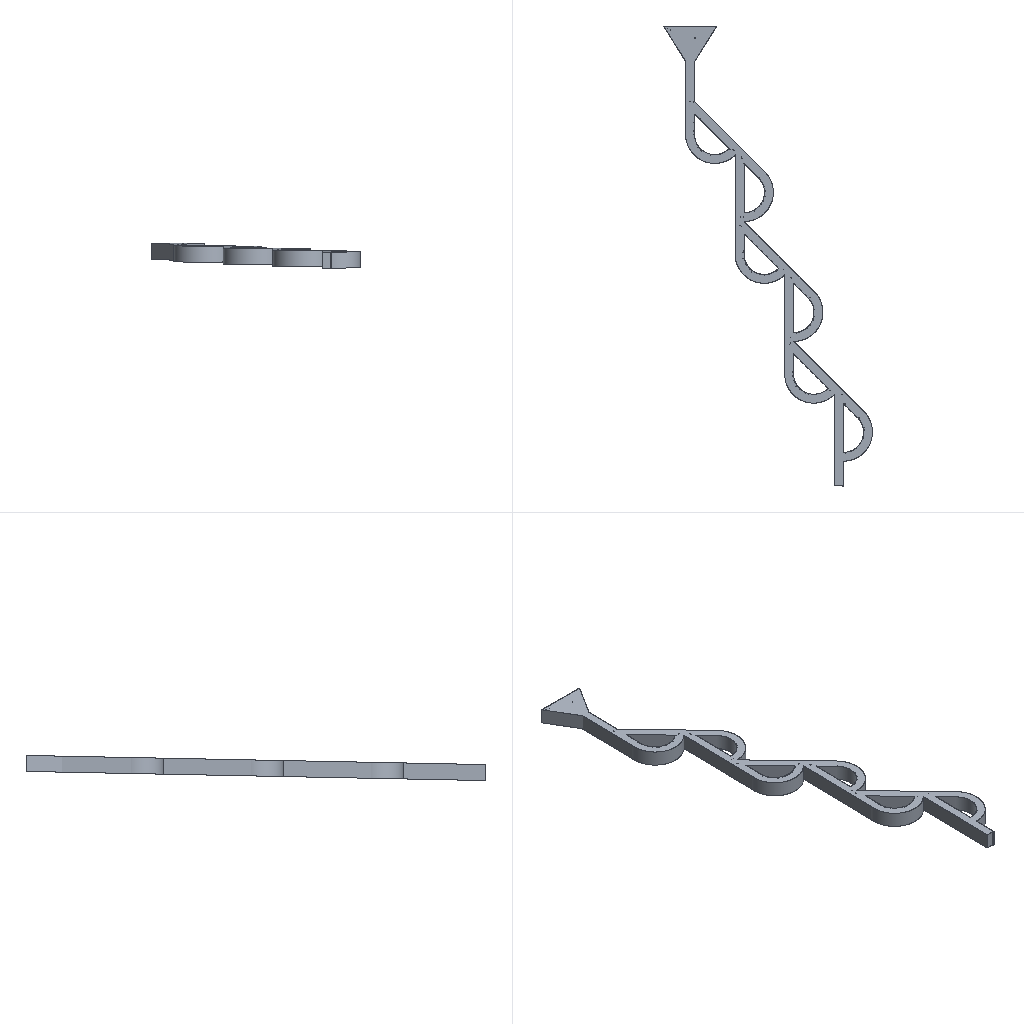Simulation study | ansys fluent
Set-up summary:
category,name,step,type,value,unit,region
solver,ansys_fluent,,Fluent 26.1.0
units,SI m-kg-s (Fluent internal),,stated,boundary values in the units shown in brackets; results in listed units
analysis,deck.cas,,cfd steady,"dimension=3D; solver=3d, dp, pbns, vof, rngke (3d, double precision, pressure-based, VOF, RNG k-epsilon); source_case=.cas"
model,Space,deck.cas,,3D
model,Time,deck.cas,,Steady
model,Viscous,deck.cas,,RNG k-epsilon turbulence model
model,Wall Treatment,deck.cas,,Standard Wall Functions
model,Heat Transfer,deck.cas,,Disabled
model,Multiphase,deck.cas,,Volume of Fluid
mesh,nodes,,,2038108
mesh,elements,,,1904760
mesh,faces,,,5845634
cell_zone,part_1 (mixture),deck.cas,fluid,material=water-liquid,,zone 3
cell_zone,part_1 (air),deck.cas,fluid,material=air,,zone 3
cell_zone,part_1 (water),deck.cas,fluid,material=water-liquid,,zone 3
material,water-liquid (fluid),,Density,998.2,kg/m^3
material,water-liquid (fluid),,Viscosity,0.001003,kg/(m s)
material,air (fluid),,Density,1.225,kg/m^3
material,air (fluid),,Viscosity,1.7894e-05,kg/(m s)
material,aluminum (solid),,Density,2719,kg/m^3
bc,out1 (mixture),deck.cas,pressure-outlet,Backflow Direction Specification Method=Normal to Boundary,,zone 7
bc,out1 (air),deck.cas,pressure-outlet,,,zone 7
bc,out1 (water),deck.cas,pressure-outlet,,,zone 7
bc,int (mixture),deck.cas,velocity-inlet,Velocity Magnitude [m/s]=0.8,,zone 6
bc,int (air),deck.cas,velocity-inlet,,,zone 6
bc,int (water),deck.cas,velocity-inlet,Volume Fraction=1,,zone 6
bc,wall-part_1 (mixture),deck.cas,wall,Wall Motion=Stationary Wall; Shear Boundary Condition=No Slip,,zone 1
bc,wall-part_1 (air),deck.cas,wall,,,zone 1
bc,wall-part_1 (water),deck.cas,wall,,,zone 1
bc,wall (mixture),deck.cas,wall,Wall Motion=Stationary Wall; Shear Boundary Condition=No Slip,,zone 8
bc,wall (air),deck.cas,wall,,,zone 8
bc,wall (water),deck.cas,wall,,,zone 8
bc,out (mixture),deck.cas,pressure-outlet,Backflow Direction Specification Method=Normal to Boundary,,zone 9
bc,out (air),deck.cas,pressure-outlet,,,zone 9
bc,out (water),deck.cas,pressure-outlet,,,zone 9
Results summary:
result,mass flow rate int,deck.cas,,8624.45,kg/s
result,mass flow rate out,deck.cas,,-200.387,kg/s
result,mass flow rate out1,deck.cas,,-7092.11,kg/s
result,mass flow rate wall,deck.cas,,-0,kg/s
result,mass flow rate wall-part_1,deck.cas,,-0,kg/s
result,mass flow rate Net,deck.cas,,1331.96,kg/s
result,wall force total wall,deck.cas,,"(6352.42, -102594, -1.38932e+06)",N
result,wall force pressure wall,deck.cas,,"(5975.7, -101478, -1.38943e+06)",N
result,wall force viscous wall,deck.cas,,"(376.726, -1115.22, 115.09)",N
result,wall force total wall-part_1,deck.cas,,"(-9514.54, 4553.51, 38.467)",N
result,wall force pressure wall-part_1,deck.cas,,"(-9548.64, 4641.52, -0.001041)",N
result,wall force viscous wall-part_1,deck.cas,,"(34.098, -88.008, 38.468)",N
result,wall force total Net,deck.cas,,"(-3162.12, -98040.1, -1.38928e+06)",N
result,wall force pressure Net,deck.cas,,"(-3572.94, -96836.8, -1.38943e+06)",N
result,wall force viscous Net,deck.cas,,"(410.824, -1203.23, 153.558)",N